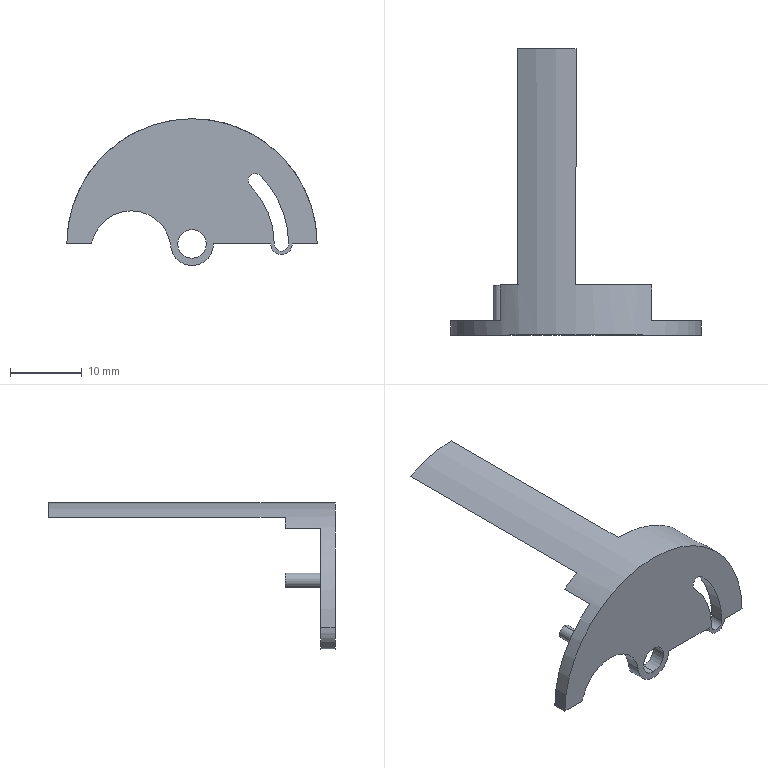Part | SolidWorks | features ICE 20, Chamfer 1, Extrusion 1 | 1 solid | 30 faces | box 35 x 40 x 20.5 mm | volume 1485 mm3 | cylinder 17 | plane 13 | commonest cylinder face diameters 2 x5 1.283 x2 3 x2 4 x2 11.161 x2 6 x1
STEP:
#1=CARTESIAN_POINT('',(-8.5,3.,4.636));
#2=VERTEX_POINT('',#1);
#3=CARTESIAN_POINT('',(-3.,3.,0.));
#4=VERTEX_POINT('',#3);
#5=CARTESIAN_POINT('',(-8.5,3.,-0.9449));
#6=DIRECTION('',(0.,1.,0.));
#7=DIRECTION('',(0.,0.,1.));
#8=AXIS2_PLACEMENT_3D('',#5,#6,#7);
#9=CIRCLE('',#8,5.581);
#10=EDGE_CURVE('',#2,#4,#9,.T.);
#11=ORIENTED_EDGE('',*,*,#10,.F.);
#12=CARTESIAN_POINT('',(-8.5,5.,4.636));
#13=VERTEX_POINT('',#12);
#14=CARTESIAN_POINT('',(-8.5,0.,4.636));
#15=DIRECTION('',(0.,1.,0.));
#16=VECTOR('',#15,1000.);
#17=LINE('',#14,#16);
#18=EDGE_CURVE('',#2,#13,#17,.T.);
#19=ORIENTED_EDGE('',*,*,#18,.T.);
#20=CARTESIAN_POINT('',(-3.,5.,0.));
#21=VERTEX_POINT('',#20);
#22=CARTESIAN_POINT('',(-8.5,5.,-0.9449));
#23=DIRECTION('',(0.,1.,0.));
#24=DIRECTION('',(0.,0.,1.));
#25=AXIS2_PLACEMENT_3D('',#22,#23,#24);
#26=CIRCLE('',#25,5.581);
#27=EDGE_CURVE('',#13,#21,#26,.T.);
#28=ORIENTED_EDGE('',*,*,#27,.T.);
#29=CARTESIAN_POINT('',(-3.,3.,0.));
#30=DIRECTION('',(0.,1.,0.));
#31=VECTOR('',#30,1000.);
#32=LINE('',#29,#31);
#33=EDGE_CURVE('',#4,#21,#32,.T.);
#34=ORIENTED_EDGE('',*,*,#33,.F.);
#35=EDGE_LOOP('',(#11,#19,#28,#34));
#36=FACE_OUTER_BOUND('',#35,.T.);
#37=CARTESIAN_POINT('',(-8.5,0.,-0.9449));
#38=DIRECTION('',(0.,1.,0.));
#39=DIRECTION('',(0.,0.,1.));
#40=AXIS2_PLACEMENT_3D('',#37,#38,#39);
#41=CYLINDRICAL_SURFACE('',#40,5.581);
#42=ADVANCED_FACE('',(#36),#41,.F.);
#43=CARTESIAN_POINT('',(-10.581,10.,7.656));
#44=VERTEX_POINT('',#43);
#45=CARTESIAN_POINT('',(-10.581,10.,5.656));
#46=VERTEX_POINT('',#45);
#47=CARTESIAN_POINT('',(-10.581,10.,6.656));
#48=DIRECTION('',(0.,1.,0.));
#49=DIRECTION('',(0.,0.,1.));
#50=AXIS2_PLACEMENT_3D('',#47,#48,#49);
#51=CIRCLE('',#50,1.);
#52=EDGE_CURVE('',#44,#46,#51,.T.);
#53=ORIENTED_EDGE('',*,*,#52,.F.);
#54=CARTESIAN_POINT('',(-10.581,5.,7.656));
#55=VERTEX_POINT('',#54);
#56=CARTESIAN_POINT('',(-10.581,10.,7.656));
#57=DIRECTION('',(0.,-1.,0.));
#58=VECTOR('',#57,1000.);
#59=LINE('',#56,#58);
#60=EDGE_CURVE('',#44,#55,#59,.T.);
#61=ORIENTED_EDGE('',*,*,#60,.T.);
#62=CARTESIAN_POINT('',(-10.581,5.,5.656));
#63=VERTEX_POINT('',#62);
#64=CARTESIAN_POINT('',(-10.581,5.,6.656));
#65=DIRECTION('',(0.,1.,0.));
#66=DIRECTION('',(0.,0.,-1.));
#67=AXIS2_PLACEMENT_3D('',#64,#65,#66);
#68=CIRCLE('',#67,1.);
#69=EDGE_CURVE('',#55,#63,#68,.T.);
#70=ORIENTED_EDGE('',*,*,#69,.T.);
#71=CARTESIAN_POINT('',(-10.581,10.,5.656));
#72=DIRECTION('',(0.,-1.,0.));
#73=VECTOR('',#72,1000.);
#74=LINE('',#71,#73);
#75=EDGE_CURVE('',#46,#63,#74,.T.);
#76=ORIENTED_EDGE('',*,*,#75,.F.);
#77=EDGE_LOOP('',(#53,#61,#70,#76));
#78=FACE_OUTER_BOUND('',#77,.T.);
#79=CARTESIAN_POINT('',(-10.581,10.,6.656));
#80=DIRECTION('',(0.,-1.,0.));
#81=DIRECTION('',(0.,0.,-1.));
#82=AXIS2_PLACEMENT_3D('',#79,#80,#81);
#83=CYLINDRICAL_SURFACE('',#82,1.);
#84=ADVANCED_FACE('',(#78),#83,.T.);
#85=CARTESIAN_POINT('',(9.546,3.,9.546));
#86=VERTEX_POINT('',#85);
#87=CARTESIAN_POINT('',(8.839,3.,9.839));
#88=VERTEX_POINT('',#87);
#89=CARTESIAN_POINT('',(8.839,3.,8.839));
#90=DIRECTION('',(0.,-1.,0.));
#91=DIRECTION('',(0.,0.,1.));
#92=AXIS2_PLACEMENT_3D('',#89,#90,#91);
#93=CIRCLE('',#92,1.);
#94=EDGE_CURVE('',#86,#88,#93,.T.);
#95=ORIENTED_EDGE('',*,*,#94,.T.);
#96=CARTESIAN_POINT('',(8.839,5.,9.839));
#97=VERTEX_POINT('',#96);
#98=CARTESIAN_POINT('',(8.839,-14.,9.839));
#99=DIRECTION('',(0.,1.,0.));
#100=VECTOR('',#99,1000.);
#101=LINE('',#98,#100);
#102=EDGE_CURVE('',#88,#97,#101,.T.);
#103=ORIENTED_EDGE('',*,*,#102,.T.);
#104=CARTESIAN_POINT('',(9.546,5.,9.546));
#105=VERTEX_POINT('',#104);
#106=CARTESIAN_POINT('',(8.839,5.,8.839));
#107=DIRECTION('',(0.,1.,0.));
#108=DIRECTION('',(0.,0.,1.));
#109=AXIS2_PLACEMENT_3D('',#106,#107,#108);
#110=CIRCLE('',#109,1.);
#111=EDGE_CURVE('',#97,#105,#110,.T.);
#112=ORIENTED_EDGE('',*,*,#111,.T.);
#113=CARTESIAN_POINT('',(9.546,-14.,9.546));
#114=DIRECTION('',(0.,1.,0.));
#115=VECTOR('',#114,1000.);
#116=LINE('',#113,#115);
#117=EDGE_CURVE('',#86,#105,#116,.T.);
#118=ORIENTED_EDGE('',*,*,#117,.F.);
#119=EDGE_LOOP('',(#95,#103,#112,#118));
#120=FACE_OUTER_BOUND('',#119,.T.);
#121=CARTESIAN_POINT('',(8.839,-14.,8.839));
#122=DIRECTION('',(0.,1.,0.));
#123=DIRECTION('',(0.,0.,1.));
#124=AXIS2_PLACEMENT_3D('',#121,#122,#123);
#125=CYLINDRICAL_SURFACE('',#124,1.);
#126=ADVANCED_FACE('',(#120),#125,.F.);
#127=CARTESIAN_POINT('',(0.,3.,2.));
#128=VERTEX_POINT('',#127);
#129=CARTESIAN_POINT('',(0.,3.,-2.));
#130=VERTEX_POINT('',#129);
#131=CARTESIAN_POINT('',(0.,3.,0.));
#132=DIRECTION('',(0.,-1.,0.));
#133=DIRECTION('',(0.,0.,1.));
#134=AXIS2_PLACEMENT_3D('',#131,#132,#133);
#135=CIRCLE('',#134,2.);
#136=EDGE_CURVE('',#128,#130,#135,.T.);
#137=ORIENTED_EDGE('',*,*,#136,.T.);
#138=CARTESIAN_POINT('',(0.,5.,-2.));
#139=VERTEX_POINT('',#138);
#140=CARTESIAN_POINT('',(0.,-1.,-2.));
#141=DIRECTION('',(0.,1.,0.));
#142=VECTOR('',#141,1000.);
#143=LINE('',#140,#142);
#144=EDGE_CURVE('',#130,#139,#143,.T.);
#145=ORIENTED_EDGE('',*,*,#144,.T.);
#146=CARTESIAN_POINT('',(0.,5.,2.));
#147=VERTEX_POINT('',#146);
#148=CARTESIAN_POINT('',(0.,5.,0.));
#149=DIRECTION('',(0.,1.,0.));
#150=DIRECTION('',(0.,0.,1.));
#151=AXIS2_PLACEMENT_3D('',#148,#149,#150);
#152=CIRCLE('',#151,2.);
#153=EDGE_CURVE('',#139,#147,#152,.T.);
#154=ORIENTED_EDGE('',*,*,#153,.T.);
#155=CARTESIAN_POINT('',(0.,-1.,2.));
#156=DIRECTION('',(0.,1.,0.));
#157=VECTOR('',#156,1000.);
#158=LINE('',#155,#157);
#159=EDGE_CURVE('',#128,#147,#158,.T.);
#160=ORIENTED_EDGE('',*,*,#159,.F.);
#161=EDGE_LOOP('',(#137,#145,#154,#160));
#162=FACE_OUTER_BOUND('',#161,.T.);
#163=CARTESIAN_POINT('',(0.,-1.,0.));
#164=DIRECTION('',(0.,1.,0.));
#165=DIRECTION('',(0.,0.,1.));
#166=AXIS2_PLACEMENT_3D('',#163,#164,#165);
#167=CYLINDRICAL_SURFACE('',#166,2.);
#168=ADVANCED_FACE('',(#162),#167,.F.);
#169=CARTESIAN_POINT('',(-17.5,3.,0.));
#170=VERTEX_POINT('',#169);
#171=CARTESIAN_POINT('',(-17.5,5.,0.));
#172=VERTEX_POINT('',#171);
#173=CARTESIAN_POINT('',(-17.5,3.,0.));
#174=DIRECTION('',(0.,1.,0.));
#175=VECTOR('',#174,1000.);
#176=LINE('',#173,#175);
#177=EDGE_CURVE('',#170,#172,#176,.T.);
#178=ORIENTED_EDGE('',*,*,#177,.F.);
#179=CARTESIAN_POINT('',(17.5,3.,0.));
#180=VERTEX_POINT('',#179);
#181=CARTESIAN_POINT('',(0.,3.,0.));
#182=DIRECTION('',(0.,1.,0.));
#183=DIRECTION('',(0.,0.,1.));
#184=AXIS2_PLACEMENT_3D('',#181,#182,#183);
#185=CIRCLE('',#184,17.5);
#186=EDGE_CURVE('',#170,#180,#185,.T.);
#187=ORIENTED_EDGE('',*,*,#186,.T.);
#188=CARTESIAN_POINT('',(17.5,5.,0.));
#189=VERTEX_POINT('',#188);
#190=CARTESIAN_POINT('',(17.5,30.,0.));
#191=DIRECTION('',(0.,1.,0.));
#192=VECTOR('',#191,1000.);
#193=LINE('',#190,#192);
#194=EDGE_CURVE('',#180,#189,#193,.T.);
#195=ORIENTED_EDGE('',*,*,#194,.T.);
#196=CARTESIAN_POINT('',(10.603,5.,13.922));
#197=VERTEX_POINT('',#196);
#198=CARTESIAN_POINT('',(0.,5.,0.));
#199=DIRECTION('',(0.,-1.,0.));
#200=DIRECTION('',(0.,0.,-1.));
#201=AXIS2_PLACEMENT_3D('',#198,#199,#200);
#202=CIRCLE('',#201,17.5);
#203=EDGE_CURVE('',#189,#197,#202,.T.);
#204=ORIENTED_EDGE('',*,*,#203,.T.);
#205=CARTESIAN_POINT('',(10.603,10.,13.922));
#206=VERTEX_POINT('',#205);
#207=CARTESIAN_POINT('',(10.603,30.,13.922));
#208=DIRECTION('',(0.,1.,0.));
#209=VECTOR('',#208,1000.);
#210=LINE('',#207,#209);
#211=EDGE_CURVE('',#197,#206,#210,.T.);
#212=ORIENTED_EDGE('',*,*,#211,.T.);
#213=CARTESIAN_POINT('',(0.,10.,17.5));
#214=VERTEX_POINT('',#213);
#215=CARTESIAN_POINT('',(0.,10.,0.));
#216=DIRECTION('',(0.,1.,0.));
#217=DIRECTION('',(0.,0.,1.));
#218=AXIS2_PLACEMENT_3D('',#215,#216,#217);
#219=CIRCLE('',#218,17.5);
#220=EDGE_CURVE('',#214,#206,#219,.T.);
#221=ORIENTED_EDGE('',*,*,#220,.F.);
#222=CARTESIAN_POINT('',(0.,43.,17.5));
#223=VERTEX_POINT('',#222);
#224=CARTESIAN_POINT('',(0.,30.,17.5));
#225=DIRECTION('',(0.,1.,0.));
#226=VECTOR('',#225,1000.);
#227=LINE('',#224,#226);
#228=EDGE_CURVE('',#214,#223,#227,.T.);
#229=ORIENTED_EDGE('',*,*,#228,.T.);
#230=CARTESIAN_POINT('',(-8.124,43.,15.5));
#231=VERTEX_POINT('',#230);
#232=CARTESIAN_POINT('',(0.,43.,0.));
#233=DIRECTION('',(0.,1.,0.));
#234=DIRECTION('',(0.,0.,1.));
#235=AXIS2_PLACEMENT_3D('',#232,#233,#234);
#236=CIRCLE('',#235,17.5);
#237=EDGE_CURVE('',#231,#223,#236,.T.);
#238=ORIENTED_EDGE('',*,*,#237,.F.);
#239=CARTESIAN_POINT('',(-8.124,10.,15.5));
#240=VERTEX_POINT('',#239);
#241=CARTESIAN_POINT('',(-8.124,30.,15.5));
#242=DIRECTION('',(0.,-1.,0.));
#243=VECTOR('',#242,1000.);
#244=LINE('',#241,#243);
#245=EDGE_CURVE('',#231,#240,#244,.T.);
#246=ORIENTED_EDGE('',*,*,#245,.T.);
#247=CARTESIAN_POINT('',(-10.603,10.,13.922));
#248=VERTEX_POINT('',#247);
#249=CARTESIAN_POINT('',(0.,10.,0.));
#250=DIRECTION('',(0.,1.,0.));
#251=DIRECTION('',(0.,0.,1.));
#252=AXIS2_PLACEMENT_3D('',#249,#250,#251);
#253=CIRCLE('',#252,17.5);
#254=EDGE_CURVE('',#248,#240,#253,.T.);
#255=ORIENTED_EDGE('',*,*,#254,.F.);
#256=CARTESIAN_POINT('',(-10.603,5.,13.922));
#257=VERTEX_POINT('',#256);
#258=CARTESIAN_POINT('',(-10.603,30.,13.922));
#259=DIRECTION('',(0.,-1.,0.));
#260=VECTOR('',#259,1000.);
#261=LINE('',#258,#260);
#262=EDGE_CURVE('',#248,#257,#261,.T.);
#263=ORIENTED_EDGE('',*,*,#262,.T.);
#264=CARTESIAN_POINT('',(0.,5.,0.));
#265=DIRECTION('',(0.,-1.,0.));
#266=DIRECTION('',(0.,0.,-1.));
#267=AXIS2_PLACEMENT_3D('',#264,#265,#266);
#268=CIRCLE('',#267,17.5);
#269=EDGE_CURVE('',#257,#172,#268,.T.);
#270=ORIENTED_EDGE('',*,*,#269,.T.);
#271=EDGE_LOOP('',(#178,#187,#195,#204,#212,#221,#229,#238,#246,#255,#263,#270));
#272=FACE_OUTER_BOUND('',#271,.T.);
#273=CARTESIAN_POINT('',(0.,30.,0.));
#274=DIRECTION('',(0.,-1.,0.));
#275=DIRECTION('',(0.,0.,-1.));
#276=AXIS2_PLACEMENT_3D('',#273,#274,#275);
#277=CYLINDRICAL_SURFACE('',#276,17.5);
#278=ADVANCED_FACE('',(#272),#277,.T.);
#279=CARTESIAN_POINT('',(0.,43.,15.5));
#280=VERTEX_POINT('',#279);
#281=CARTESIAN_POINT('',(0.,10.,15.5));
#282=VERTEX_POINT('',#281);
#283=CARTESIAN_POINT('',(0.,30.,15.5));
#284=DIRECTION('',(0.,-1.,0.));
#285=VECTOR('',#284,1000.);
#286=LINE('',#283,#285);
#287=EDGE_CURVE('',#280,#282,#286,.T.);
#288=ORIENTED_EDGE('',*,*,#287,.T.);
#289=CARTESIAN_POINT('',(-8.124,10.,15.5));
#290=DIRECTION('',(1.,0.,0.));
#291=VECTOR('',#290,1000.);
#292=LINE('',#289,#291);
#293=EDGE_CURVE('',#240,#282,#292,.T.);
#294=ORIENTED_EDGE('',*,*,#293,.F.);
#295=ORIENTED_EDGE('',*,*,#245,.F.);
#296=CARTESIAN_POINT('',(0.,43.,15.5));
#297=DIRECTION('',(-1.,0.,0.));
#298=VECTOR('',#297,1000.);
#299=LINE('',#296,#298);
#300=EDGE_CURVE('',#280,#231,#299,.T.);
#301=ORIENTED_EDGE('',*,*,#300,.F.);
#302=EDGE_LOOP('',(#288,#294,#295,#301));
#303=FACE_OUTER_BOUND('',#302,.T.);
#304=CARTESIAN_POINT('',(-17.5,30.,15.5));
#305=DIRECTION('',(0.,0.,1.));
#306=DIRECTION('',(0.,-1.,0.));
#307=AXIS2_PLACEMENT_3D('',#304,#305,#306);
#308=PLANE('',#307);
#309=ADVANCED_FACE('',(#303),#308,.F.);
#310=ORIENTED_EDGE('',*,*,#228,.F.);
#311=CARTESIAN_POINT('',(0.,10.,15.5));
#312=DIRECTION('',(0.,0.,1.));
#313=VECTOR('',#312,1000.);
#314=LINE('',#311,#313);
#315=EDGE_CURVE('',#282,#214,#314,.T.);
#316=ORIENTED_EDGE('',*,*,#315,.F.);
#317=ORIENTED_EDGE('',*,*,#287,.F.);
#318=CARTESIAN_POINT('',(0.,43.,17.5));
#319=DIRECTION('',(0.,0.,-1.));
#320=VECTOR('',#319,1000.);
#321=LINE('',#318,#320);
#322=EDGE_CURVE('',#223,#280,#321,.T.);
#323=ORIENTED_EDGE('',*,*,#322,.F.);
#324=EDGE_LOOP('',(#310,#316,#317,#323));
#325=FACE_OUTER_BOUND('',#324,.T.);
#326=CARTESIAN_POINT('',(0.,30.,17.5));
#327=DIRECTION('',(-1.,0.,0.));
#328=DIRECTION('',(0.,-1.,0.));
#329=AXIS2_PLACEMENT_3D('',#326,#327,#328);
#330=PLANE('',#329);
#331=ADVANCED_FACE('',(#325),#330,.F.);
#332=CARTESIAN_POINT('',(14.,3.,0.));
#333=VERTEX_POINT('',#332);
#334=CARTESIAN_POINT('',(14.,5.,0.));
#335=VERTEX_POINT('',#334);
#336=CARTESIAN_POINT('',(14.,3.,0.));
#337=DIRECTION('',(0.,1.,0.));
#338=VECTOR('',#337,1000.);
#339=LINE('',#336,#338);
#340=EDGE_CURVE('',#333,#335,#339,.T.);
#341=ORIENTED_EDGE('',*,*,#340,.T.);
#342=CARTESIAN_POINT('',(14.,5.,0.));
#343=DIRECTION('',(1.,0.,0.));
#344=VECTOR('',#343,1000.);
#345=LINE('',#342,#344);
#346=EDGE_CURVE('',#335,#189,#345,.T.);
#347=ORIENTED_EDGE('',*,*,#346,.T.);
#348=ORIENTED_EDGE('',*,*,#194,.F.);
#349=CARTESIAN_POINT('',(14.,3.,0.));
#350=DIRECTION('',(1.,0.,0.));
#351=VECTOR('',#350,1000.);
#352=LINE('',#349,#351);
#353=EDGE_CURVE('',#333,#180,#352,.T.);
#354=ORIENTED_EDGE('',*,*,#353,.F.);
#355=EDGE_LOOP('',(#341,#347,#348,#354));
#356=FACE_OUTER_BOUND('',#355,.T.);
#357=CARTESIAN_POINT('',(14.,3.,0.));
#358=DIRECTION('',(0.,0.,1.));
#359=DIRECTION('',(1.,0.,0.));
#360=AXIS2_PLACEMENT_3D('',#357,#358,#359);
#361=PLANE('',#360);
#362=ADVANCED_FACE('',(#356),#361,.F.);
#363=CARTESIAN_POINT('',(11.,3.,0.));
#364=VERTEX_POINT('',#363);
#365=CARTESIAN_POINT('',(11.,5.,0.));
#366=VERTEX_POINT('',#365);
#367=CARTESIAN_POINT('',(11.,3.,0.));
#368=DIRECTION('',(0.,1.,0.));
#369=VECTOR('',#368,1000.);
#370=LINE('',#367,#369);
#371=EDGE_CURVE('',#364,#366,#370,.T.);
#372=ORIENTED_EDGE('',*,*,#371,.T.);
#373=CARTESIAN_POINT('',(12.5,5.,0.));
#374=DIRECTION('',(0.,-1.,0.));
#375=DIRECTION('',(0.,0.,-1.));
#376=AXIS2_PLACEMENT_3D('',#373,#374,#375);
#377=CIRCLE('',#376,1.5);
#378=EDGE_CURVE('',#366,#335,#377,.T.);
#379=ORIENTED_EDGE('',*,*,#378,.T.);
#380=ORIENTED_EDGE('',*,*,#340,.F.);
#381=CARTESIAN_POINT('',(12.5,3.,0.));
#382=DIRECTION('',(0.,-1.,0.));
#383=DIRECTION('',(0.,0.,1.));
#384=AXIS2_PLACEMENT_3D('',#381,#382,#383);
#385=CIRCLE('',#384,1.5);
#386=EDGE_CURVE('',#364,#333,#385,.T.);
#387=ORIENTED_EDGE('',*,*,#386,.F.);
#388=EDGE_LOOP('',(#372,#379,#380,#387));
#389=FACE_OUTER_BOUND('',#388,.T.);
#390=CARTESIAN_POINT('',(12.5,3.,0.));
#391=DIRECTION('',(0.,1.,0.));
#392=DIRECTION('',(0.,0.,1.));
#393=AXIS2_PLACEMENT_3D('',#390,#391,#392);
#394=CYLINDRICAL_SURFACE('',#393,1.5);
#395=ADVANCED_FACE('',(#389),#394,.T.);
#396=CARTESIAN_POINT('',(3.,3.,0.));
#397=VERTEX_POINT('',#396);
#398=CARTESIAN_POINT('',(3.,5.,0.));
#399=VERTEX_POINT('',#398);
#400=CARTESIAN_POINT('',(3.,3.,0.));
#401=DIRECTION('',(0.,1.,0.));
#402=VECTOR('',#401,1000.);
#403=LINE('',#400,#402);
#404=EDGE_CURVE('',#397,#399,#403,.T.);
#405=ORIENTED_EDGE('',*,*,#404,.T.);
#406=CARTESIAN_POINT('',(3.,5.,0.));
#407=DIRECTION('',(1.,0.,0.));
#408=VECTOR('',#407,1000.);
#409=LINE('',#406,#408);
#410=EDGE_CURVE('',#399,#366,#409,.T.);
#411=ORIENTED_EDGE('',*,*,#410,.T.);
#412=ORIENTED_EDGE('',*,*,#371,.F.);
#413=CARTESIAN_POINT('',(3.,3.,0.));
#414=DIRECTION('',(1.,0.,0.));
#415=VECTOR('',#414,1000.);
#416=LINE('',#413,#415);
#417=EDGE_CURVE('',#397,#364,#416,.T.);
#418=ORIENTED_EDGE('',*,*,#417,.F.);
#419=EDGE_LOOP('',(#405,#411,#412,#418));
#420=FACE_OUTER_BOUND('',#419,.T.);
#421=CARTESIAN_POINT('',(3.,3.,0.));
#422=DIRECTION('',(0.,0.,1.));
#423=DIRECTION('',(1.,0.,0.));
#424=AXIS2_PLACEMENT_3D('',#421,#422,#423);
#425=PLANE('',#424);
#426=ADVANCED_FACE('',(#420),#425,.F.);
#427=ORIENTED_EDGE('',*,*,#33,.T.);
#428=CARTESIAN_POINT('',(0.,5.,0.));
#429=DIRECTION('',(0.,-1.,0.));
#430=DIRECTION('',(0.,0.,-1.));
#431=AXIS2_PLACEMENT_3D('',#428,#429,#430);
#432=CIRCLE('',#431,3.);
#433=EDGE_CURVE('',#21,#399,#432,.T.);
#434=ORIENTED_EDGE('',*,*,#433,.T.);
#435=ORIENTED_EDGE('',*,*,#404,.F.);
#436=CARTESIAN_POINT('',(0.,3.,0.));
#437=DIRECTION('',(0.,-1.,0.));
#438=DIRECTION('',(0.,0.,1.));
#439=AXIS2_PLACEMENT_3D('',#436,#437,#438);
#440=CIRCLE('',#439,3.);
#441=EDGE_CURVE('',#4,#397,#440,.T.);
#442=ORIENTED_EDGE('',*,*,#441,.F.);
#443=EDGE_LOOP('',(#427,#434,#435,#442));
#444=FACE_OUTER_BOUND('',#443,.T.);
#445=CARTESIAN_POINT('',(0.,3.,0.));
#446=DIRECTION('',(0.,1.,0.));
#447=DIRECTION('',(0.,0.,1.));
#448=AXIS2_PLACEMENT_3D('',#445,#446,#447);
#449=CYLINDRICAL_SURFACE('',#448,3.);
#450=ADVANCED_FACE('',(#444),#449,.T.);
#451=CARTESIAN_POINT('',(-14.,5.,0.));
#452=VERTEX_POINT('',#451);
#453=CARTESIAN_POINT('',(-17.5,5.,0.));
#454=DIRECTION('',(1.,0.,0.));
#455=VECTOR('',#454,1000.);
#456=LINE('',#453,#455);
#457=EDGE_CURVE('',#172,#452,#456,.T.);
#458=ORIENTED_EDGE('',*,*,#457,.T.);
#459=CARTESIAN_POINT('',(-14.,3.,0.));
#460=VERTEX_POINT('',#459);
#461=CARTESIAN_POINT('',(-14.,3.,0.));
#462=DIRECTION('',(0.,-1.,0.));
#463=VECTOR('',#462,1000.);
#464=LINE('',#461,#463);
#465=EDGE_CURVE('',#452,#460,#464,.T.);
#466=ORIENTED_EDGE('',*,*,#465,.T.);
#467=CARTESIAN_POINT('',(-17.5,3.,0.));
#468=DIRECTION('',(1.,0.,0.));
#469=VECTOR('',#468,1000.);
#470=LINE('',#467,#469);
#471=EDGE_CURVE('',#170,#460,#470,.T.);
#472=ORIENTED_EDGE('',*,*,#471,.F.);
#473=ORIENTED_EDGE('',*,*,#177,.T.);
#474=EDGE_LOOP('',(#458,#466,#472,#473));
#475=FACE_OUTER_BOUND('',#474,.T.);
#476=CARTESIAN_POINT('',(-17.5,3.,0.));
#477=DIRECTION('',(0.,0.,1.));
#478=DIRECTION('',(1.,0.,0.));
#479=AXIS2_PLACEMENT_3D('',#476,#477,#478);
#480=PLANE('',#479);
#481=ADVANCED_FACE('',(#475),#480,.F.);
#482=ORIENTED_EDGE('',*,*,#262,.F.);
#483=CARTESIAN_POINT('',(10.603,10.,13.922));
#484=DIRECTION('',(-1.,0.,0.));
#485=VECTOR('',#484,1000.);
#486=LINE('',#483,#485);
#487=EDGE_CURVE('',#206,#248,#486,.T.);
#488=ORIENTED_EDGE('',*,*,#487,.F.);
#489=ORIENTED_EDGE('',*,*,#211,.F.);
#490=CARTESIAN_POINT('',(-17.5,5.,13.922));
#491=DIRECTION('',(1.,0.,0.));
#492=VECTOR('',#491,1000.);
#493=LINE('',#490,#492);
#494=EDGE_CURVE('',#257,#197,#493,.T.);
#495=ORIENTED_EDGE('',*,*,#494,.F.);
#496=EDGE_LOOP('',(#482,#488,#489,#495));
#497=FACE_OUTER_BOUND('',#496,.T.);
#498=CARTESIAN_POINT('',(-17.5,7.,13.922));
#499=DIRECTION('',(0.,0.,1.));
#500=DIRECTION('',(1.,0.,0.));
#501=AXIS2_PLACEMENT_3D('',#498,#499,#500);
#502=PLANE('',#501);
#503=ADVANCED_FACE('',(#497),#502,.F.);
#504=CARTESIAN_POINT('',(-10.581,5.,6.656));
#505=DIRECTION('',(0.,1.,0.));
#506=DIRECTION('',(0.,0.,-1.));
#507=AXIS2_PLACEMENT_3D('',#504,#505,#506);
#508=CIRCLE('',#507,1.);
#509=EDGE_CURVE('',#63,#55,#508,.T.);
#510=ORIENTED_EDGE('',*,*,#509,.F.);
#511=ORIENTED_EDGE('',*,*,#69,.F.);
#512=EDGE_LOOP('',(#510,#511));
#513=FACE_BOUND('',#512,.T.);
#514=CARTESIAN_POINT('',(13.5,5.,0.));
#515=VERTEX_POINT('',#514);
#516=CARTESIAN_POINT('',(0.,5.,0.));
#517=DIRECTION('',(0.,1.,0.));
#518=DIRECTION('',(0.,0.,1.));
#519=AXIS2_PLACEMENT_3D('',#516,#517,#518);
#520=CIRCLE('',#519,13.5);
#521=EDGE_CURVE('',#105,#515,#520,.T.);
#522=ORIENTED_EDGE('',*,*,#521,.F.);
#523=ORIENTED_EDGE('',*,*,#111,.F.);
#524=CARTESIAN_POINT('',(8.132,5.,8.132));
#525=VERTEX_POINT('',#524);
#526=CARTESIAN_POINT('',(8.839,5.,8.839));
#527=DIRECTION('',(0.,1.,0.));
#528=DIRECTION('',(0.,0.,1.));
#529=AXIS2_PLACEMENT_3D('',#526,#527,#528);
#530=CIRCLE('',#529,1.);
#531=EDGE_CURVE('',#525,#97,#530,.T.);
#532=ORIENTED_EDGE('',*,*,#531,.F.);
#533=CARTESIAN_POINT('',(11.5,5.,0.));
#534=VERTEX_POINT('',#533);
#535=CARTESIAN_POINT('',(0.,5.,0.));
#536=DIRECTION('',(0.,-1.,0.));
#537=DIRECTION('',(0.,0.,1.));
#538=AXIS2_PLACEMENT_3D('',#535,#536,#537);
#539=CIRCLE('',#538,11.5);
#540=EDGE_CURVE('',#534,#525,#539,.T.);
#541=ORIENTED_EDGE('',*,*,#540,.F.);
#542=CARTESIAN_POINT('',(12.5,5.,0.));
#543=DIRECTION('',(0.,1.,0.));
#544=DIRECTION('',(0.,0.,1.));
#545=AXIS2_PLACEMENT_3D('',#542,#543,#544);
#546=CIRCLE('',#545,1.);
#547=EDGE_CURVE('',#515,#534,#546,.T.);
#548=ORIENTED_EDGE('',*,*,#547,.F.);
#549=EDGE_LOOP('',(#522,#523,#532,#541,#548));
#550=FACE_BOUND('',#549,.T.);
#551=CARTESIAN_POINT('',(0.,5.,0.));
#552=DIRECTION('',(0.,1.,0.));
#553=DIRECTION('',(0.,0.,1.));
#554=AXIS2_PLACEMENT_3D('',#551,#552,#553);
#555=CIRCLE('',#554,2.);
#556=EDGE_CURVE('',#147,#139,#555,.T.);
#557=ORIENTED_EDGE('',*,*,#556,.F.);
#558=ORIENTED_EDGE('',*,*,#153,.F.);
#559=EDGE_LOOP('',(#557,#558));
#560=FACE_BOUND('',#559,.T.);
#561=ORIENTED_EDGE('',*,*,#433,.F.);
#562=ORIENTED_EDGE('',*,*,#27,.F.);
#563=CARTESIAN_POINT('',(-13.841,5.,0.6712));
#564=VERTEX_POINT('',#563);
#565=CARTESIAN_POINT('',(-8.5,5.,-0.9449));
#566=DIRECTION('',(0.,1.,0.));
#567=DIRECTION('',(0.,0.,1.));
#568=AXIS2_PLACEMENT_3D('',#565,#566,#567);
#569=CIRCLE('',#568,5.581);
#570=EDGE_CURVE('',#564,#13,#569,.T.);
#571=ORIENTED_EDGE('',*,*,#570,.F.);
#572=CARTESIAN_POINT('',(-12.5,5.,0.));
#573=DIRECTION('',(0.,-1.,0.));
#574=DIRECTION('',(0.,0.,-1.));
#575=AXIS2_PLACEMENT_3D('',#572,#573,#574);
#576=CIRCLE('',#575,1.5);
#577=EDGE_CURVE('',#564,#452,#576,.T.);
#578=ORIENTED_EDGE('',*,*,#577,.T.);
#579=ORIENTED_EDGE('',*,*,#457,.F.);
#580=ORIENTED_EDGE('',*,*,#269,.F.);
#581=ORIENTED_EDGE('',*,*,#494,.T.);
#582=ORIENTED_EDGE('',*,*,#203,.F.);
#583=ORIENTED_EDGE('',*,*,#346,.F.);
#584=ORIENTED_EDGE('',*,*,#378,.F.);
#585=ORIENTED_EDGE('',*,*,#410,.F.);
#586=EDGE_LOOP('',(#561,#562,#571,#578,#579,#580,#581,#582,#583,#584,#585));
#587=FACE_OUTER_BOUND('',#586,.T.);
#588=CARTESIAN_POINT('',(-17.5,5.,13.922));
#589=DIRECTION('',(0.,-1.,0.));
#590=DIRECTION('',(0.,0.,-1.));
#591=AXIS2_PLACEMENT_3D('',#588,#589,#590);
#592=PLANE('',#591);
#593=ADVANCED_FACE('',(#513,#550,#560,#587),#592,.F.);
#594=ORIENTED_EDGE('',*,*,#144,.F.);
#595=CARTESIAN_POINT('',(0.,3.,0.));
#596=DIRECTION('',(0.,-1.,0.));
#597=DIRECTION('',(0.,0.,1.));
#598=AXIS2_PLACEMENT_3D('',#595,#596,#597);
#599=CIRCLE('',#598,2.);
#600=EDGE_CURVE('',#130,#128,#599,.T.);
#601=ORIENTED_EDGE('',*,*,#600,.T.);
#602=ORIENTED_EDGE('',*,*,#159,.T.);
#603=ORIENTED_EDGE('',*,*,#556,.T.);
#604=EDGE_LOOP('',(#594,#601,#602,#603));
#605=FACE_OUTER_BOUND('',#604,.T.);
#606=CARTESIAN_POINT('',(0.,-1.,0.));
#607=DIRECTION('',(0.,1.,0.));
#608=DIRECTION('',(0.,0.,1.));
#609=AXIS2_PLACEMENT_3D('',#606,#607,#608);
#610=CYLINDRICAL_SURFACE('',#609,2.);
#611=ADVANCED_FACE('',(#605),#610,.F.);
#612=ORIENTED_EDGE('',*,*,#102,.F.);
#613=CARTESIAN_POINT('',(8.132,3.,8.132));
#614=VERTEX_POINT('',#613);
#615=CARTESIAN_POINT('',(8.839,3.,8.839));
#616=DIRECTION('',(0.,-1.,0.));
#617=DIRECTION('',(0.,0.,1.));
#618=AXIS2_PLACEMENT_3D('',#615,#616,#617);
#619=CIRCLE('',#618,1.);
#620=EDGE_CURVE('',#88,#614,#619,.T.);
#621=ORIENTED_EDGE('',*,*,#620,.T.);
#622=CARTESIAN_POINT('',(8.132,-14.,8.132));
#623=DIRECTION('',(0.,1.,0.));
#624=VECTOR('',#623,1000.);
#625=LINE('',#622,#624);
#626=EDGE_CURVE('',#614,#525,#625,.T.);
#627=ORIENTED_EDGE('',*,*,#626,.T.);
#628=ORIENTED_EDGE('',*,*,#531,.T.);
#629=EDGE_LOOP('',(#612,#621,#627,#628));
#630=FACE_OUTER_BOUND('',#629,.T.);
#631=CARTESIAN_POINT('',(8.839,-14.,8.839));
#632=DIRECTION('',(0.,1.,0.));
#633=DIRECTION('',(0.,0.,1.));
#634=AXIS2_PLACEMENT_3D('',#631,#632,#633);
#635=CYLINDRICAL_SURFACE('',#634,1.);
#636=ADVANCED_FACE('',(#630),#635,.F.);
#637=ORIENTED_EDGE('',*,*,#626,.F.);
#638=CARTESIAN_POINT('',(11.5,3.,0.));
#639=VERTEX_POINT('',#638);
#640=CARTESIAN_POINT('',(0.,3.,0.));
#641=DIRECTION('',(0.,1.,0.));
#642=DIRECTION('',(0.,0.,1.));
#643=AXIS2_PLACEMENT_3D('',#640,#641,#642);
#644=CIRCLE('',#643,11.5);
#645=EDGE_CURVE('',#614,#639,#644,.T.);
#646=ORIENTED_EDGE('',*,*,#645,.T.);
#647=CARTESIAN_POINT('',(11.5,-14.,0.));
#648=DIRECTION('',(0.,1.,0.));
#649=VECTOR('',#648,1000.);
#650=LINE('',#647,#649);
#651=EDGE_CURVE('',#639,#534,#650,.T.);
#652=ORIENTED_EDGE('',*,*,#651,.T.);
#653=ORIENTED_EDGE('',*,*,#540,.T.);
#654=EDGE_LOOP('',(#637,#646,#652,#653));
#655=FACE_OUTER_BOUND('',#654,.T.);
#656=CARTESIAN_POINT('',(0.,-14.,0.));
#657=DIRECTION('',(0.,1.,0.));
#658=DIRECTION('',(0.,0.,1.));
#659=AXIS2_PLACEMENT_3D('',#656,#657,#658);
#660=CYLINDRICAL_SURFACE('',#659,11.5);
#661=ADVANCED_FACE('',(#655),#660,.T.);
#662=ORIENTED_EDGE('',*,*,#651,.F.);
#663=CARTESIAN_POINT('',(13.5,3.,0.));
#664=VERTEX_POINT('',#663);
#665=CARTESIAN_POINT('',(12.5,3.,0.));
#666=DIRECTION('',(0.,-1.,0.));
#667=DIRECTION('',(0.,0.,1.));
#668=AXIS2_PLACEMENT_3D('',#665,#666,#667);
#669=CIRCLE('',#668,1.);
#670=EDGE_CURVE('',#639,#664,#669,.T.);
#671=ORIENTED_EDGE('',*,*,#670,.T.);
#672=CARTESIAN_POINT('',(13.5,-14.,0.));
#673=DIRECTION('',(0.,1.,0.));
#674=VECTOR('',#673,1000.);
#675=LINE('',#672,#674);
#676=EDGE_CURVE('',#664,#515,#675,.T.);
#677=ORIENTED_EDGE('',*,*,#676,.T.);
#678=ORIENTED_EDGE('',*,*,#547,.T.);
#679=EDGE_LOOP('',(#662,#671,#677,#678));
#680=FACE_OUTER_BOUND('',#679,.T.);
#681=CARTESIAN_POINT('',(12.5,-14.,0.));
#682=DIRECTION('',(0.,1.,0.));
#683=DIRECTION('',(0.,0.,1.));
#684=AXIS2_PLACEMENT_3D('',#681,#682,#683);
#685=CYLINDRICAL_SURFACE('',#684,1.);
#686=ADVANCED_FACE('',(#680),#685,.F.);
#687=ORIENTED_EDGE('',*,*,#676,.F.);
#688=CARTESIAN_POINT('',(0.,3.,0.));
#689=DIRECTION('',(0.,-1.,0.));
#690=DIRECTION('',(0.,0.,1.));
#691=AXIS2_PLACEMENT_3D('',#688,#689,#690);
#692=CIRCLE('',#691,13.5);
#693=EDGE_CURVE('',#664,#86,#692,.T.);
#694=ORIENTED_EDGE('',*,*,#693,.T.);
#695=ORIENTED_EDGE('',*,*,#117,.T.);
#696=ORIENTED_EDGE('',*,*,#521,.T.);
#697=EDGE_LOOP('',(#687,#694,#695,#696));
#698=FACE_OUTER_BOUND('',#697,.T.);
#699=CARTESIAN_POINT('',(0.,-14.,0.));
#700=DIRECTION('',(0.,1.,0.));
#701=DIRECTION('',(0.,0.,1.));
#702=AXIS2_PLACEMENT_3D('',#699,#700,#701);
#703=CYLINDRICAL_SURFACE('',#702,13.5);
#704=ADVANCED_FACE('',(#698),#703,.F.);
#705=ORIENTED_EDGE('',*,*,#693,.F.);
#706=ORIENTED_EDGE('',*,*,#670,.F.);
#707=ORIENTED_EDGE('',*,*,#645,.F.);
#708=ORIENTED_EDGE('',*,*,#620,.F.);
#709=ORIENTED_EDGE('',*,*,#94,.F.);
#710=EDGE_LOOP('',(#705,#706,#707,#708,#709));
#711=FACE_BOUND('',#710,.T.);
#712=ORIENTED_EDGE('',*,*,#136,.F.);
#713=ORIENTED_EDGE('',*,*,#600,.F.);
#714=EDGE_LOOP('',(#712,#713));
#715=FACE_BOUND('',#714,.T.);
#716=CARTESIAN_POINT('',(-13.841,3.,0.6712));
#717=VERTEX_POINT('',#716);
#718=CARTESIAN_POINT('',(-12.5,3.,0.));
#719=DIRECTION('',(0.,1.,0.));
#720=DIRECTION('',(0.,0.,1.));
#721=AXIS2_PLACEMENT_3D('',#718,#719,#720);
#722=CIRCLE('',#721,1.5);
#723=EDGE_CURVE('',#460,#717,#722,.T.);
#724=ORIENTED_EDGE('',*,*,#723,.T.);
#725=CARTESIAN_POINT('',(-8.5,3.,-0.9449));
#726=DIRECTION('',(0.,1.,0.));
#727=DIRECTION('',(0.,0.,1.));
#728=AXIS2_PLACEMENT_3D('',#725,#726,#727);
#729=CIRCLE('',#728,5.581);
#730=EDGE_CURVE('',#717,#2,#729,.T.);
#731=ORIENTED_EDGE('',*,*,#730,.T.);
#732=ORIENTED_EDGE('',*,*,#10,.T.);
#733=ORIENTED_EDGE('',*,*,#441,.T.);
#734=ORIENTED_EDGE('',*,*,#417,.T.);
#735=ORIENTED_EDGE('',*,*,#386,.T.);
#736=ORIENTED_EDGE('',*,*,#353,.T.);
#737=ORIENTED_EDGE('',*,*,#186,.F.);
#738=ORIENTED_EDGE('',*,*,#471,.T.);
#739=EDGE_LOOP('',(#724,#731,#732,#733,#734,#735,#736,#737,#738));
#740=FACE_OUTER_BOUND('',#739,.T.);
#741=CARTESIAN_POINT('',(0.,3.,0.));
#742=DIRECTION('',(0.,1.,0.));
#743=DIRECTION('',(0.,0.,1.));
#744=AXIS2_PLACEMENT_3D('',#741,#742,#743);
#745=PLANE('',#744);
#746=ADVANCED_FACE('',(#711,#715,#740),#745,.F.);
#747=ORIENTED_EDGE('',*,*,#220,.T.);
#748=ORIENTED_EDGE('',*,*,#487,.T.);
#749=ORIENTED_EDGE('',*,*,#254,.T.);
#750=ORIENTED_EDGE('',*,*,#293,.T.);
#751=ORIENTED_EDGE('',*,*,#315,.T.);
#752=EDGE_LOOP('',(#747,#748,#749,#750,#751));
#753=FACE_OUTER_BOUND('',#752,.T.);
#754=CARTESIAN_POINT('',(0.,10.,0.));
#755=DIRECTION('',(0.,1.,0.));
#756=DIRECTION('',(0.,0.,1.));
#757=AXIS2_PLACEMENT_3D('',#754,#755,#756);
#758=PLANE('',#757);
#759=ADVANCED_FACE('',(#753),#758,.T.);
#760=ORIENTED_EDGE('',*,*,#237,.T.);
#761=ORIENTED_EDGE('',*,*,#322,.T.);
#762=ORIENTED_EDGE('',*,*,#300,.T.);
#763=EDGE_LOOP('',(#760,#761,#762));
#764=FACE_OUTER_BOUND('',#763,.T.);
#765=CARTESIAN_POINT('',(0.,43.,0.));
#766=DIRECTION('',(0.,1.,0.));
#767=DIRECTION('',(0.,0.,1.));
#768=AXIS2_PLACEMENT_3D('',#765,#766,#767);
#769=PLANE('',#768);
#770=ADVANCED_FACE('',(#764),#769,.T.);
#771=ORIENTED_EDGE('',*,*,#577,.F.);
#772=CARTESIAN_POINT('',(-13.841,2.5,0.6712));
#773=DIRECTION('',(0.,-1.,0.));
#774=VECTOR('',#773,1000.);
#775=LINE('',#772,#774);
#776=EDGE_CURVE('',#564,#717,#775,.T.);
#777=ORIENTED_EDGE('',*,*,#776,.T.);
#778=ORIENTED_EDGE('',*,*,#723,.F.);
#779=ORIENTED_EDGE('',*,*,#465,.F.);
#780=EDGE_LOOP('',(#771,#777,#778,#779));
#781=FACE_OUTER_BOUND('',#780,.T.);
#782=CARTESIAN_POINT('',(-12.5,3.,0.));
#783=DIRECTION('',(0.,1.,0.));
#784=DIRECTION('',(0.,0.,1.));
#785=AXIS2_PLACEMENT_3D('',#782,#783,#784);
#786=CYLINDRICAL_SURFACE('',#785,1.5);
#787=ADVANCED_FACE('',(#781),#786,.F.);
#788=ORIENTED_EDGE('',*,*,#60,.F.);
#789=CARTESIAN_POINT('',(-10.581,10.,6.656));
#790=DIRECTION('',(0.,1.,0.));
#791=DIRECTION('',(0.,0.,1.));
#792=AXIS2_PLACEMENT_3D('',#789,#790,#791);
#793=CIRCLE('',#792,1.);
#794=EDGE_CURVE('',#46,#44,#793,.T.);
#795=ORIENTED_EDGE('',*,*,#794,.F.);
#796=ORIENTED_EDGE('',*,*,#75,.T.);
#797=ORIENTED_EDGE('',*,*,#509,.T.);
#798=EDGE_LOOP('',(#788,#795,#796,#797));
#799=FACE_OUTER_BOUND('',#798,.T.);
#800=CARTESIAN_POINT('',(-10.581,10.,6.656));
#801=DIRECTION('',(0.,-1.,0.));
#802=DIRECTION('',(0.,0.,-1.));
#803=AXIS2_PLACEMENT_3D('',#800,#801,#802);
#804=CYLINDRICAL_SURFACE('',#803,1.);
#805=ADVANCED_FACE('',(#799),#804,.T.);
#806=ORIENTED_EDGE('',*,*,#794,.T.);
#807=ORIENTED_EDGE('',*,*,#52,.T.);
#808=EDGE_LOOP('',(#806,#807));
#809=FACE_OUTER_BOUND('',#808,.T.);
#810=CARTESIAN_POINT('',(-10.581,10.,6.656));
#811=DIRECTION('',(0.,1.,0.));
#812=DIRECTION('',(0.,0.,1.));
#813=AXIS2_PLACEMENT_3D('',#810,#811,#812);
#814=PLANE('',#813);
#815=ADVANCED_FACE('',(#809),#814,.T.);
#816=ORIENTED_EDGE('',*,*,#18,.F.);
#817=ORIENTED_EDGE('',*,*,#730,.F.);
#818=ORIENTED_EDGE('',*,*,#776,.F.);
#819=ORIENTED_EDGE('',*,*,#570,.T.);
#820=EDGE_LOOP('',(#816,#817,#818,#819));
#821=FACE_OUTER_BOUND('',#820,.T.);
#822=CARTESIAN_POINT('',(-8.5,0.,-0.9449));
#823=DIRECTION('',(0.,1.,0.));
#824=DIRECTION('',(0.,0.,1.));
#825=AXIS2_PLACEMENT_3D('',#822,#823,#824);
#826=CYLINDRICAL_SURFACE('',#825,5.581);
#827=ADVANCED_FACE('',(#821),#826,.F.);
#828=CLOSED_SHELL('',(#42,#84,#126,#168,#278,#309,#331,#362,#395,#426,#450,#481,#503,#593,#611,#636,#661,#686,#704,#746,#759,#770,#787,#805,#815,#827));
#829=CARTESIAN_POINT('',(-1.034,30.,17.165));
#830=VERTEX_POINT('',#829);
#831=CARTESIAN_POINT('',(-1.034,30.,15.882));
#832=VERTEX_POINT('',#831);
#833=CARTESIAN_POINT('',(-1.034,30.,16.523));
#834=DIRECTION('',(0.,-1.,0.));
#835=DIRECTION('',(0.,0.,1.));
#836=AXIS2_PLACEMENT_3D('',#833,#834,#835);
#837=CIRCLE('',#836,0.6413);
#838=EDGE_CURVE('',#830,#832,#837,.T.);
#839=ORIENTED_EDGE('',*,*,#838,.F.);
#840=CARTESIAN_POINT('',(-1.034,29.5,17.165));
#841=VERTEX_POINT('',#840);
#842=CARTESIAN_POINT('',(-1.034,30.,17.165));
#843=DIRECTION('',(0.,-1.,0.));
#844=VECTOR('',#843,1000.);
#845=LINE('',#842,#844);
#846=EDGE_CURVE('',#830,#841,#845,.T.);
#847=ORIENTED_EDGE('',*,*,#846,.T.);
#848=CARTESIAN_POINT('',(-1.034,29.5,15.882));
#849=VERTEX_POINT('',#848);
#850=CARTESIAN_POINT('',(-1.034,29.5,16.523));
#851=DIRECTION('',(0.,1.,0.));
#852=DIRECTION('',(0.,0.,1.));
#853=AXIS2_PLACEMENT_3D('',#850,#851,#852);
#854=CIRCLE('',#853,0.6413);
#855=EDGE_CURVE('',#849,#841,#854,.T.);
#856=ORIENTED_EDGE('',*,*,#855,.F.);
#857=CARTESIAN_POINT('',(-1.034,30.,15.882));
#858=DIRECTION('',(0.,-1.,0.));
#859=VECTOR('',#858,1000.);
#860=LINE('',#857,#859);
#861=EDGE_CURVE('',#832,#849,#860,.T.);
#862=ORIENTED_EDGE('',*,*,#861,.F.);
#863=EDGE_LOOP('',(#839,#847,#856,#862));
#864=FACE_OUTER_BOUND('',#863,.T.);
#865=CARTESIAN_POINT('',(-1.034,30.,16.523));
#866=DIRECTION('',(0.,-1.,0.));
#867=DIRECTION('',(0.,0.,-1.));
#868=AXIS2_PLACEMENT_3D('',#865,#866,#867);
#869=CYLINDRICAL_SURFACE('',#868,0.6413);
#870=ADVANCED_FACE('',(#864),#869,.F.);
#871=CARTESIAN_POINT('',(-1.034,30.,16.523));
#872=DIRECTION('',(0.,-1.,0.));
#873=DIRECTION('',(0.,0.,1.));
#874=AXIS2_PLACEMENT_3D('',#871,#872,#873);
#875=CIRCLE('',#874,0.6413);
#876=EDGE_CURVE('',#832,#830,#875,.T.);
#877=ORIENTED_EDGE('',*,*,#876,.T.);
#878=ORIENTED_EDGE('',*,*,#838,.T.);
#879=EDGE_LOOP('',(#877,#878));
#880=FACE_OUTER_BOUND('',#879,.T.);
#881=CARTESIAN_POINT('',(0.,30.,0.));
#882=DIRECTION('',(0.,1.,0.));
#883=DIRECTION('',(0.,0.,1.));
#884=AXIS2_PLACEMENT_3D('',#881,#882,#883);
#885=PLANE('',#884);
#886=ADVANCED_FACE('',(#880),#885,.F.);
#887=ORIENTED_EDGE('',*,*,#855,.T.);
#888=CARTESIAN_POINT('',(-1.034,29.5,16.523));
#889=DIRECTION('',(0.,1.,0.));
#890=DIRECTION('',(0.,0.,1.));
#891=AXIS2_PLACEMENT_3D('',#888,#889,#890);
#892=CIRCLE('',#891,0.6413);
#893=EDGE_CURVE('',#841,#849,#892,.T.);
#894=ORIENTED_EDGE('',*,*,#893,.T.);
#895=EDGE_LOOP('',(#887,#894));
#896=FACE_OUTER_BOUND('',#895,.T.);
#897=CARTESIAN_POINT('',(-1.034,29.5,16.523));
#898=DIRECTION('',(0.,1.,0.));
#899=DIRECTION('',(0.,0.,1.));
#900=AXIS2_PLACEMENT_3D('',#897,#898,#899);
#901=PLANE('',#900);
#902=ADVANCED_FACE('',(#896),#901,.T.);
#903=ORIENTED_EDGE('',*,*,#846,.F.);
#904=ORIENTED_EDGE('',*,*,#876,.F.);
#905=ORIENTED_EDGE('',*,*,#861,.T.);
#906=ORIENTED_EDGE('',*,*,#893,.F.);
#907=EDGE_LOOP('',(#903,#904,#905,#906));
#908=FACE_OUTER_BOUND('',#907,.T.);
#909=CARTESIAN_POINT('',(-1.034,30.,16.523));
#910=DIRECTION('',(0.,-1.,0.));
#911=DIRECTION('',(0.,0.,-1.));
#912=AXIS2_PLACEMENT_3D('',#909,#910,#911);
#913=CYLINDRICAL_SURFACE('',#912,0.6413);
#914=ADVANCED_FACE('',(#908),#913,.F.);
#915=CLOSED_SHELL('',(#870,#886,#902,#914));
#916=ORIENTED_CLOSED_SHELL('',*,#915,.F.);
#917=BREP_WITH_VOIDS('',#828,(#916));
#918=CARTESIAN_POINT('',(0.,0.,0.));
#919=DIRECTION('',(0.,0.,1.));
#920=DIRECTION('',(1.,0.,0.));
#921=AXIS2_PLACEMENT_3D('',#918,#919,#920);
#922=(LENGTH_UNIT()NAMED_UNIT(*)SI_UNIT(.MILLI.,.METRE.));
#923=UNCERTAINTY_MEASURE_WITH_UNIT(LENGTH_MEASURE(0.00001),#922,'','');
#924=(NAMED_UNIT(*)PLANE_ANGLE_UNIT()SI_UNIT($,.RADIAN.));
#925=(NAMED_UNIT(*)SI_UNIT($,.STERADIAN.)SOLID_ANGLE_UNIT());
#926=(GEOMETRIC_REPRESENTATION_CONTEXT(3)GLOBAL_UNCERTAINTY_ASSIGNED_CONTEXT((#923))GLOBAL_UNIT_ASSIGNED_CONTEXT((#922,#924,#925))REPRESENTATION_CONTEXT('',''));
#927=ADVANCED_BREP_SHAPE_REPRESENTATION('',(#917,#921),#926);